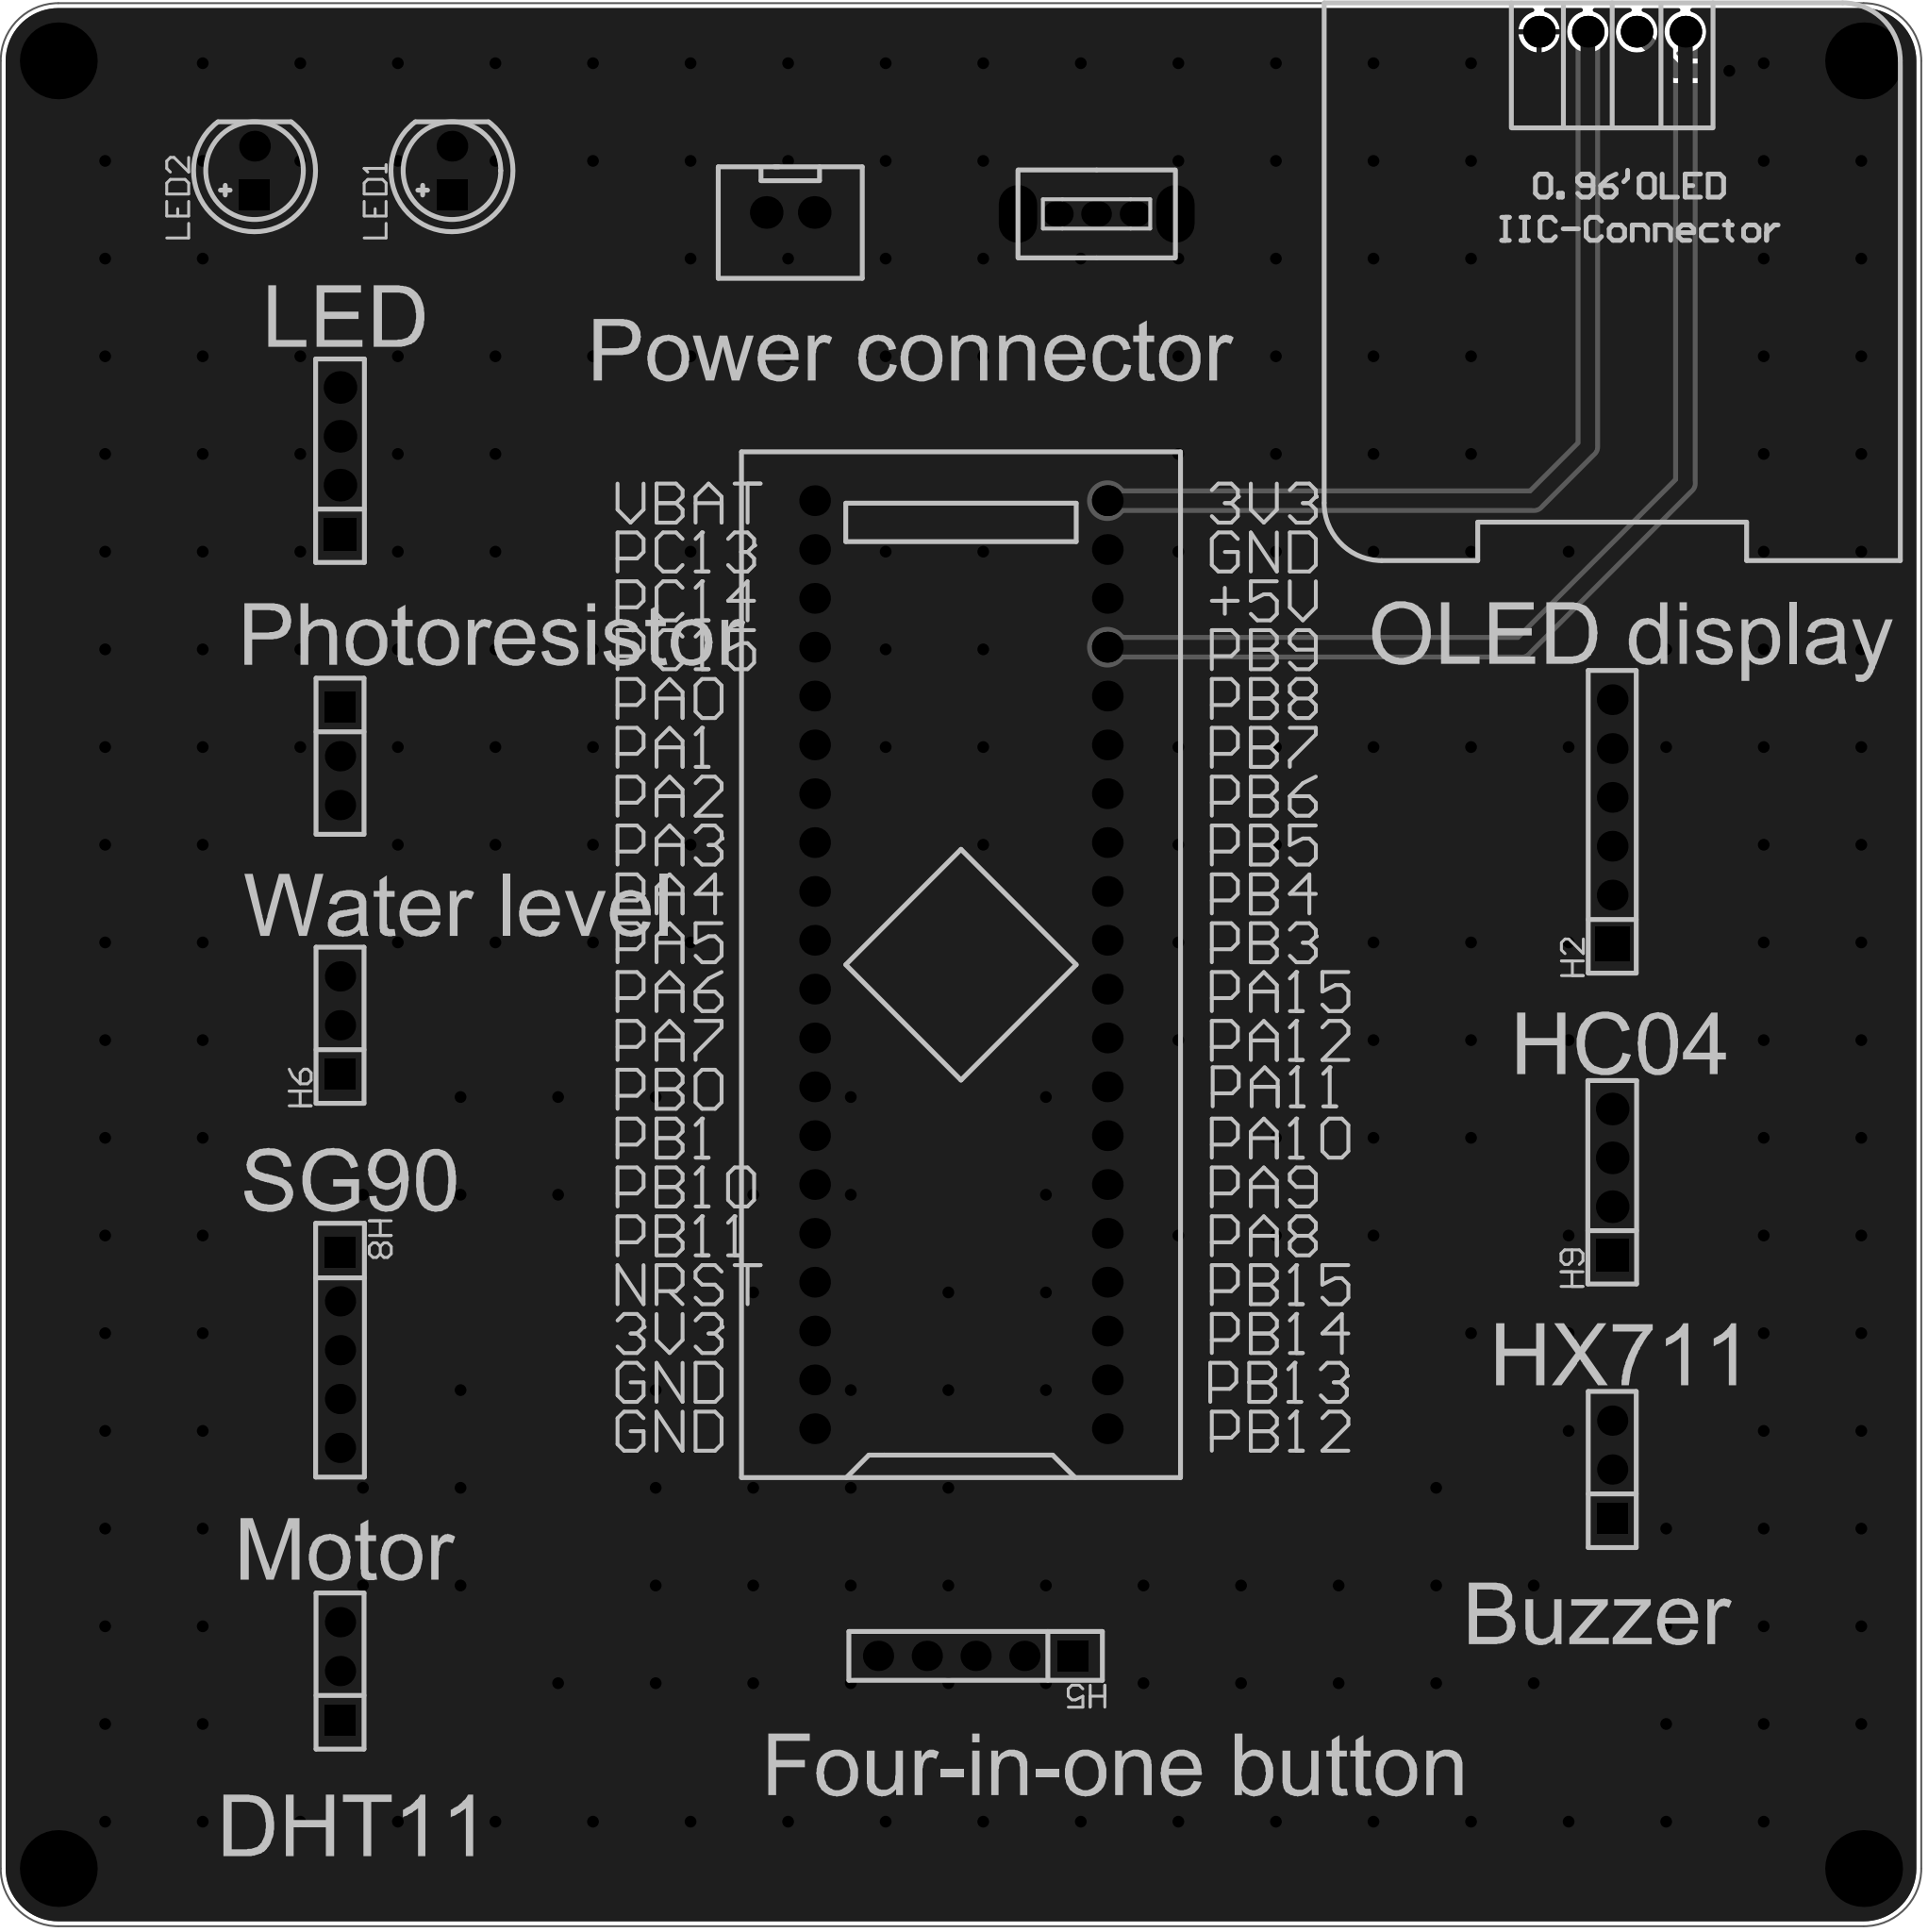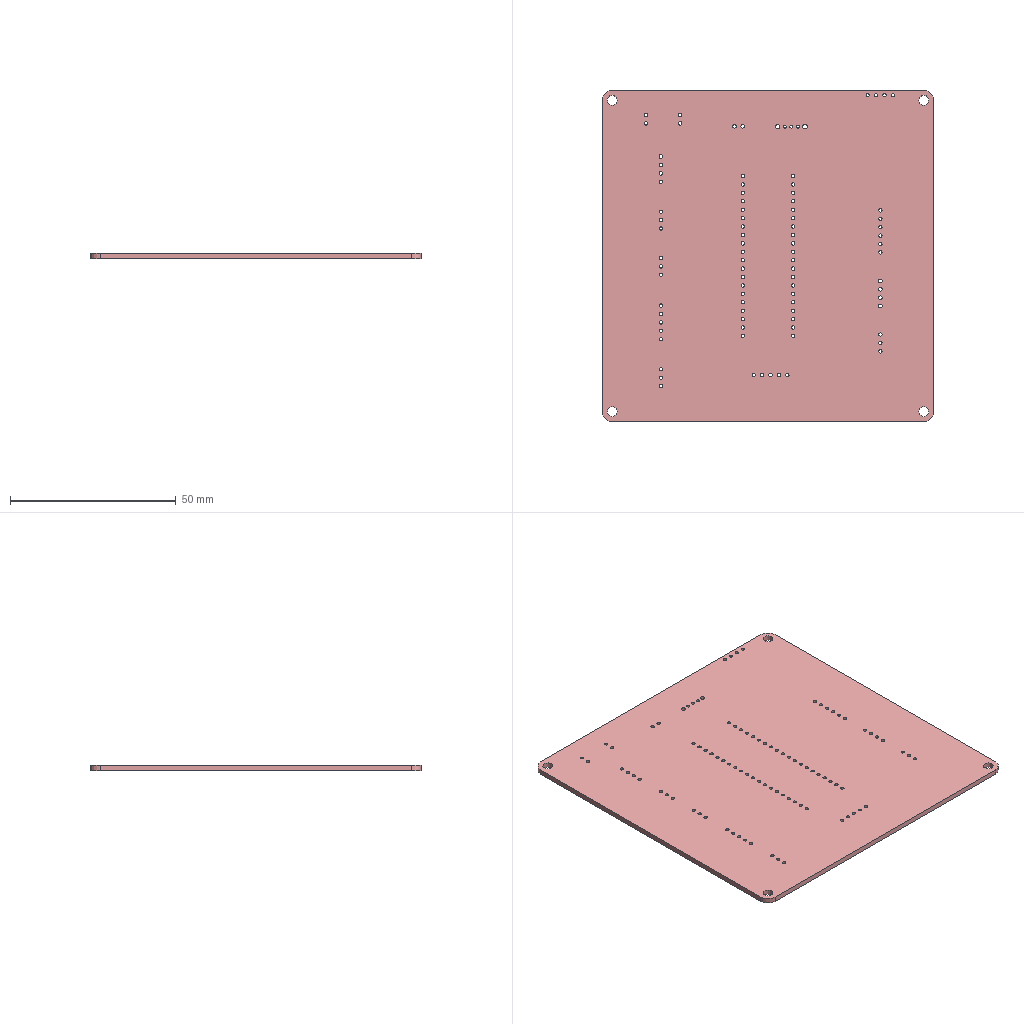Circuit board layout | Altium Designer | box 100 x 100 x 1.6 mm
Layer stack:
# Altium Designer layer stack of  (unit mm; dielectric type: 0 none, 1 core, 2 prepreg, 3 surface material)
index,name,kind,layer,copper_thickness_mm,dielectric_type,dielectric_thickness_mm,dielectric_material,dielectric_constant
0,Top Paste Mask Layer,other,,,,,,
1,Top Silkscreen Layer,other,,,,,,
2,Top Solder Mask Layer,dielectric,,,3,0.01,,3.3
3,Top Layer,copper,Top Layer,0.035,,,,
4,Dielectric1,dielectric,,,3,1.51,FR4,4.5
5,Bottom Layer,copper,Bottom Layer,0.035,,,,
6,Bottom Solder Mask Layer,dielectric,,,3,0.01,,3.3
7,Bottom Silkscreen Layer,other,,,,,,
8,Bottom Paste Mask Layer,other,,,,,,
# drill layer pairs: low layer,high layer
drill_pair,Top Layer,Bottom Layer
Part placement:
Designator,Comment,Layer,Footprint,Center-X(mm),Center-Y(mm),Rotation
U1,STM32F103C8T6-Card,TopLayer,CONN-TH_L53.3-W22.9_STM32F103C8T6-CARD,141.351,130.937,90
OLED1,,TopLayer,0.96OLED_4P,175.26,179.451,0
H12,,TopLayer,HDR-TH_3P-P2.54-V-F,109.018,141.778,270
CN4,XH2.54*2P_Straight,TopLayer,CONN-TH_2P-P2.50-XH2.54-2P,132.461,170.053,0
SW5,,TopLayer,拨动开关,148.417,169.978,0
H1,,TopLayer,HDR-TH_3P-P2.54-V-F,175.26,104.688,90
H3,,TopLayer,HDR-TH_3P-P2.54-V-F,109.018,94.207,90
H4,,TopLayer,HDR-TH_4P-P2.54-V-F,109.018,157.144,90
H2,,TopLayer,HDR-TH_6P-P2.54-V-F,175.26,138.368,90
H5,,TopLayer,HDR-TH_5P-P2.54-V-F,142.113,94.996,180
H6,,TopLayer,HDR-TH_3P-P2.54-V-F,109.018,127.788,90
H8,,TopLayer,HDR-TH_5P-P2.54-V-F,109.018,110.892,270
H9,,TopLayer,HDR-TH_4P-P2.54-V-F,175.26,119.623,90
LED1,,TopLayer,LED-TH_5mm,114.846,172.229,90
LED2,,TopLayer,LED-TH_5mm,104.567,172.229,90
Pad and via stacks:
# Altium Designer via and pad stacks of  (unit mm). Each distinct definition once, with the count of objects using it.
# via: kind,start_layer,end_layer,hole_mm,diameter_mm,mode(0 simple;1 top-mid-bottom;2 full stack),diameter_per_layer,count,example_net
# pad: kind,layer,hole_mm,hole_type(0 round;1 square;2 slot),plating,top_size,top_shape(1 round;2 rect;3 octagon;9 rounded rect),mid_size,bottom_size,mode,footprint,size_per_layer,count,example
pad,Multi-Layer,3,0,plated,4x4,1,4x4,4x4,0,,,4,1
pad,Multi-Layer,1,0,plated,1.6x1.6,1,1.6x1.6,1.6x1.6,0,CONN-TH_L53.3-W22.9_STM32F103C8T6-CARD,,40,U1.1
pad,Multi-Layer,1,0,plated,1.65x1.65,1,1.65x1.65,1.65x1.65,0,0.96OLED_4P,,4,OLED1.4
pad,Multi-Layer,1.02,0,plated,1.575x1.575,1,1.575x1.575,1.575x1.575,0,HDR-TH_3P-P2.54-V-F,,8,H12.3
pad,Multi-Layer,1.02,0,plated,1.575x1.575,2,1.575x1.575,1.575x1.575,0,HDR-TH_3P-P2.54-V-F,,4,H12.1
pad,Multi-Layer,1.05,0,plated,1.7x1.7,1,1.7x1.7,1.7x1.7,0,CONN-TH_2P-P2.50-XH2.54-2P,,2,CN4.2
pad,Multi-Layer,0.8992,0,plated,1.6x1.3,1,1.6x1.3,1.6x1.3,0,\u00B2\u00A6\u00B6\u00AF\u00BF\u00AA\u00B9\u00D8,,3,SW5.1
pad,Multi-Layer,1.3,0,plated,3x1.999,1,3x1.999,3x1.999,0,\u00B2\u00A6\u00B6\u00AF\u00BF\u00AA\u00B9\u00D8,,2,SW5.4
pad,Multi-Layer,1.1,0,plated,1.7x1.7,2,1.7x1.7,1.7x1.7,0,HDR-TH_4P-P2.54-V-F,,2,H4.1
pad,Multi-Layer,1.1,0,plated,1.7x1.7,1,1.7x1.7,1.7x1.7,0,HDR-TH_4P-P2.54-V-F,,6,H4.2
pad,Multi-Layer,1.02,0,plated,1.6x1.6,1,1.6x1.6,1.6x1.6,0,HDR-TH_6P-P2.54-V-F,,5,H2.6
pad,Multi-Layer,1.02,0,plated,1.8x1.8,2,1.8x1.8,1.8x1.8,0,HDR-TH_6P-P2.54-V-F,,1,H2.1
pad,Multi-Layer,1.02,0,plated,1.575x1.575,1,1.575x1.575,1.575x1.575,0,HDR-TH_5P-P2.54-V-F,,8,H5.5
pad,Multi-Layer,1.02,0,plated,1.575x1.575,2,1.575x1.575,1.575x1.575,0,HDR-TH_5P-P2.54-V-F,,2,H5.1
pad,Multi-Layer,1,0,plated,1.6x1.6,2,1.6x1.6,1.6x1.6,0,LED-TH_5mm,,2,LED1.1
pad,Multi-Layer,1,0,plated,1.6x1.6,1,1.6x1.6,1.6x1.6,0,LED-TH_5mm,,2,LED1.2
via,Top Layer,Bottom Layer,0.3048,0.61,0,,254,PB8
Copper pours:
name,layer,net,type(0 solid;1 hatched;2 none)
Bottom Layer-GND,Bottom Layer,GND,0
Top Layer-GND,Top Layer,GND,0
Design rules, without the lines most boards share:
# Altium Designer design rules of  (exported by Altium Designer, unit mm)
# columns: name | kind | enabled | priority | scope1 | scope2 | descriptor | typed fields (field=value)
Copper_copperRegion_copperThickness1oz | 0 | disabled | 4 | All | All | Clearance Constraint (Gap=5.984mil) (Disabled)(All),(All) | gap=0.152
Copper_copperRegion_copperThickness1oz_1 | 63 | disabled | 4 | All | All | Board Clearance Constraint (Gap=0mil) (Disabled)(All) |
Copper_copperRegion_Copper_copperRegion | 0 | disabled | 5 | All | All | Clearance Constraint (Gap=5.984mil) (Disabled)(All),(All) | gap=0.152
Copper_copperRegion_Copper_copperRegion_1 | 63 | disabled | 5 | All | All | Board Clearance Constraint (Gap=0mil) (Disabled)(All) |
copperThickness1oz | 0 | enabled | 6 | All | All | Clearance Constraint (Gap=5.984mil) (All),(All) | gap=0.152
copperThickness1oz_1 | 63 | enabled | 6 | All | All | Board Clearance Constraint (Gap=0mil) (All) |
copperRegion_copperThickness1oz | 20 | disabled | 1 | All | All | Polygon Connect Rule(Relief Connect )(Conductor Width=10mil) (Relief Angle=90 Angle) (Entries=4) (Air Gap Width=10mil) (Disabled)(All),(All) | connect_style(0=relief,1=direct,2=none)=0 relief_conductor_width=0.254 relief_entries=4
copperRegion_Copper_copperRegion | 20 | disabled | 2 | All | All | Polygon Connect Rule(Relief Connect )(Conductor Width=10mil) (Relief Angle=90 Angle) (Entries=4) (Air Gap Width=10mil) (Disabled)(All),(All) | connect_style(0=relief,1=direct,2=none)=0 relief_conductor_width=0.254 relief_entries=4
copperRegion | 20 | enabled | 3 | All | All | Polygon Connect Rule(Relief Connect )(Conductor Width=10mil) (Relief Angle=90 Angle) (Entries=4) (Air Gap Width=10mil) (All),(All) | connect_style(0=relief,1=direct,2=none)=0 relief_conductor_width=0.254 relief_entries=4